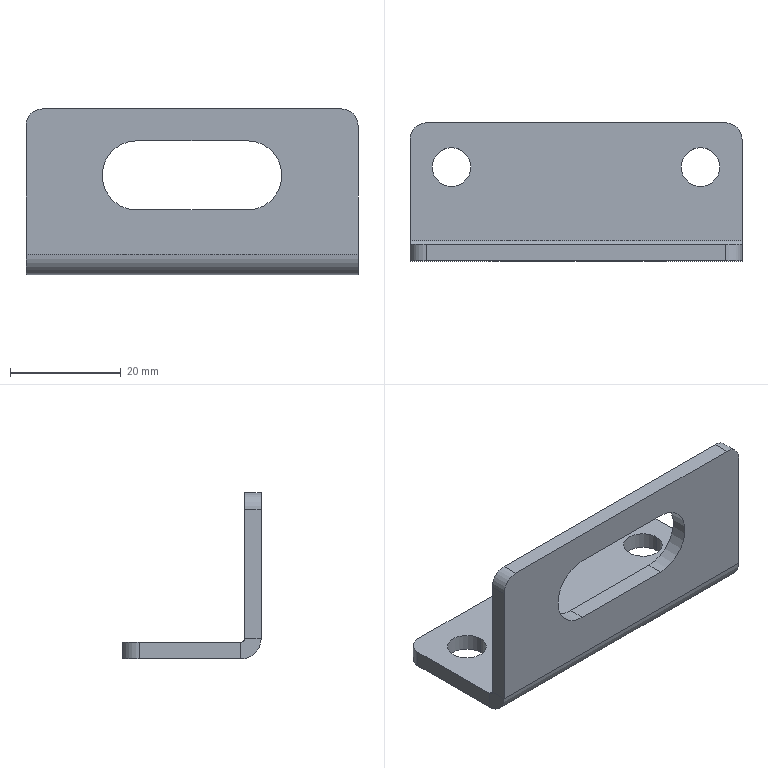Part | SolidWorks | features BaseBody 1 | 1 solid | 26 faces | box 60 x 25 x 30 mm | volume 7815 mm3 | plane 14 | cylinder 12 | commonest cylinder face diameters 6 x4 7 x4 12.5 x2 1.473 x1 7.473 x1
STEP:
#1=CARTESIAN_POINT('',(-26.,4.5,-3.));
#2=VERTEX_POINT('',#1);
#3=CARTESIAN_POINT('',(-19.,4.5,-3.));
#4=VERTEX_POINT('',#3);
#5=CARTESIAN_POINT('',(-22.5,4.5,-3.));
#6=DIRECTION('',(0.,0.,1.));
#7=DIRECTION('',(1.,0.,0.));
#8=AXIS2_PLACEMENT_3D('',#5,#6,#7);
#9=CIRCLE('',#8,3.5);
#10=EDGE_CURVE('',#2,#4,#9,.T.);
#11=ORIENTED_EDGE('',*,*,#10,.F.);
#12=CARTESIAN_POINT('',(-26.,4.5,0.));
#13=VERTEX_POINT('',#12);
#14=CARTESIAN_POINT('',(-26.,4.5,0.));
#15=DIRECTION('',(0.,0.,1.));
#16=VECTOR('',#15,1000.);
#17=LINE('',#14,#16);
#18=EDGE_CURVE('',#2,#13,#17,.T.);
#19=ORIENTED_EDGE('',*,*,#18,.T.);
#20=CARTESIAN_POINT('',(-19.,4.5,0.));
#21=VERTEX_POINT('',#20);
#22=CARTESIAN_POINT('',(-22.5,4.5,0.));
#23=DIRECTION('',(0.,0.,1.));
#24=DIRECTION('',(1.,0.,0.));
#25=AXIS2_PLACEMENT_3D('',#22,#23,#24);
#26=CIRCLE('',#25,3.5);
#27=EDGE_CURVE('',#13,#21,#26,.T.);
#28=ORIENTED_EDGE('',*,*,#27,.T.);
#29=CARTESIAN_POINT('',(-19.,4.5,0.));
#30=DIRECTION('',(0.,0.,1.));
#31=VECTOR('',#30,1000.);
#32=LINE('',#29,#31);
#33=EDGE_CURVE('',#4,#21,#32,.T.);
#34=ORIENTED_EDGE('',*,*,#33,.F.);
#35=EDGE_LOOP('',(#11,#19,#28,#34));
#36=FACE_OUTER_BOUND('',#35,.T.);
#37=CARTESIAN_POINT('',(-22.5,4.5,0.));
#38=DIRECTION('',(0.,0.,1.));
#39=DIRECTION('',(1.,0.,0.));
#40=AXIS2_PLACEMENT_3D('',#37,#38,#39);
#41=CYLINDRICAL_SURFACE('',#40,3.5);
#42=ADVANCED_FACE('',(#36),#41,.F.);
#43=CARTESIAN_POINT('',(19.,4.5,-3.));
#44=VERTEX_POINT('',#43);
#45=CARTESIAN_POINT('',(26.,4.5,-3.));
#46=VERTEX_POINT('',#45);
#47=CARTESIAN_POINT('',(22.5,4.5,-3.));
#48=DIRECTION('',(0.,0.,1.));
#49=DIRECTION('',(1.,0.,0.));
#50=AXIS2_PLACEMENT_3D('',#47,#48,#49);
#51=CIRCLE('',#50,3.5);
#52=EDGE_CURVE('',#44,#46,#51,.T.);
#53=ORIENTED_EDGE('',*,*,#52,.F.);
#54=CARTESIAN_POINT('',(19.,4.5,0.));
#55=VERTEX_POINT('',#54);
#56=CARTESIAN_POINT('',(19.,4.5,0.));
#57=DIRECTION('',(0.,0.,1.));
#58=VECTOR('',#57,1000.);
#59=LINE('',#56,#58);
#60=EDGE_CURVE('',#44,#55,#59,.T.);
#61=ORIENTED_EDGE('',*,*,#60,.T.);
#62=CARTESIAN_POINT('',(26.,4.5,0.));
#63=VERTEX_POINT('',#62);
#64=CARTESIAN_POINT('',(22.5,4.5,0.));
#65=DIRECTION('',(0.,0.,1.));
#66=DIRECTION('',(1.,0.,0.));
#67=AXIS2_PLACEMENT_3D('',#64,#65,#66);
#68=CIRCLE('',#67,3.5);
#69=EDGE_CURVE('',#55,#63,#68,.T.);
#70=ORIENTED_EDGE('',*,*,#69,.T.);
#71=CARTESIAN_POINT('',(26.,4.5,0.));
#72=DIRECTION('',(0.,0.,1.));
#73=VECTOR('',#72,1000.);
#74=LINE('',#71,#73);
#75=EDGE_CURVE('',#46,#63,#74,.T.);
#76=ORIENTED_EDGE('',*,*,#75,.F.);
#77=EDGE_LOOP('',(#53,#61,#70,#76));
#78=FACE_OUTER_BOUND('',#77,.T.);
#79=CARTESIAN_POINT('',(22.5,4.5,0.));
#80=DIRECTION('',(0.,0.,1.));
#81=DIRECTION('',(1.,0.,0.));
#82=AXIS2_PLACEMENT_3D('',#79,#80,#81);
#83=CYLINDRICAL_SURFACE('',#82,3.5);
#84=ADVANCED_FACE('',(#78),#83,.F.);
#85=CARTESIAN_POINT('',(-10.,-9.5,8.75));
#86=VERTEX_POINT('',#85);
#87=CARTESIAN_POINT('',(-10.,-12.5,8.75));
#88=VERTEX_POINT('',#87);
#89=CARTESIAN_POINT('',(-10.,-9.5,8.75));
#90=DIRECTION('',(0.,-1.,0.));
#91=VECTOR('',#90,1000.);
#92=LINE('',#89,#91);
#93=EDGE_CURVE('',#86,#88,#92,.T.);
#94=ORIENTED_EDGE('',*,*,#93,.F.);
#95=CARTESIAN_POINT('',(-10.,-9.5,21.25));
#96=VERTEX_POINT('',#95);
#97=CARTESIAN_POINT('',(-10.,-9.5,15.));
#98=DIRECTION('',(0.,1.,0.));
#99=DIRECTION('',(0.,0.,1.));
#100=AXIS2_PLACEMENT_3D('',#97,#98,#99);
#101=CIRCLE('',#100,6.25);
#102=EDGE_CURVE('',#86,#96,#101,.T.);
#103=ORIENTED_EDGE('',*,*,#102,.T.);
#104=CARTESIAN_POINT('',(-10.,-12.5,21.25));
#105=VERTEX_POINT('',#104);
#106=CARTESIAN_POINT('',(-10.,-9.5,21.25));
#107=DIRECTION('',(0.,-1.,0.));
#108=VECTOR('',#107,1000.);
#109=LINE('',#106,#108);
#110=EDGE_CURVE('',#96,#105,#109,.T.);
#111=ORIENTED_EDGE('',*,*,#110,.T.);
#112=CARTESIAN_POINT('',(-10.,-12.5,15.));
#113=DIRECTION('',(0.,1.,0.));
#114=DIRECTION('',(0.,0.,1.));
#115=AXIS2_PLACEMENT_3D('',#112,#113,#114);
#116=CIRCLE('',#115,6.25);
#117=EDGE_CURVE('',#88,#105,#116,.T.);
#118=ORIENTED_EDGE('',*,*,#117,.F.);
#119=EDGE_LOOP('',(#94,#103,#111,#118));
#120=FACE_OUTER_BOUND('',#119,.T.);
#121=CARTESIAN_POINT('',(-10.,-9.5,15.));
#122=DIRECTION('',(0.,1.,0.));
#123=DIRECTION('',(0.,0.,1.));
#124=AXIS2_PLACEMENT_3D('',#121,#122,#123);
#125=CYLINDRICAL_SURFACE('',#124,6.25);
#126=ADVANCED_FACE('',(#120),#125,.F.);
#127=CARTESIAN_POINT('',(30.,-8.763,-3.));
#128=VERTEX_POINT('',#127);
#129=CARTESIAN_POINT('',(30.,9.5,-3.));
#130=VERTEX_POINT('',#129);
#131=CARTESIAN_POINT('',(30.,12.5,-3.));
#132=DIRECTION('',(0.,1.,0.));
#133=VECTOR('',#132,1000.);
#134=LINE('',#131,#133);
#135=EDGE_CURVE('',#128,#130,#134,.T.);
#136=ORIENTED_EDGE('',*,*,#135,.T.);
#137=CARTESIAN_POINT('',(30.,9.5,0.));
#138=VERTEX_POINT('',#137);
#139=CARTESIAN_POINT('',(30.,9.5,-3.));
#140=DIRECTION('',(0.,0.,1.));
#141=VECTOR('',#140,1000.);
#142=LINE('',#139,#141);
#143=EDGE_CURVE('',#130,#138,#142,.T.);
#144=ORIENTED_EDGE('',*,*,#143,.T.);
#145=CARTESIAN_POINT('',(30.,-8.763,0.));
#146=VERTEX_POINT('',#145);
#147=CARTESIAN_POINT('',(30.,12.5,0.));
#148=DIRECTION('',(0.,1.,0.));
#149=VECTOR('',#148,1000.);
#150=LINE('',#147,#149);
#151=EDGE_CURVE('',#146,#138,#150,.T.);
#152=ORIENTED_EDGE('',*,*,#151,.F.);
#153=CARTESIAN_POINT('',(30.,-8.763,0.));
#154=DIRECTION('',(0.,0.,-1.));
#155=VECTOR('',#154,1000.);
#156=LINE('',#153,#155);
#157=EDGE_CURVE('',#146,#128,#156,.T.);
#158=ORIENTED_EDGE('',*,*,#157,.T.);
#159=EDGE_LOOP('',(#136,#144,#152,#158));
#160=FACE_OUTER_BOUND('',#159,.T.);
#161=CARTESIAN_POINT('',(30.,12.5,-3.));
#162=DIRECTION('',(1.,0.,0.));
#163=DIRECTION('',(0.,1.,0.));
#164=AXIS2_PLACEMENT_3D('',#161,#162,#163);
#165=PLANE('',#164);
#166=ADVANCED_FACE('',(#160),#165,.T.);
#167=CARTESIAN_POINT('',(-22.5,4.5,-3.));
#168=DIRECTION('',(0.,0.,1.));
#169=DIRECTION('',(1.,0.,0.));
#170=AXIS2_PLACEMENT_3D('',#167,#168,#169);
#171=CIRCLE('',#170,3.5);
#172=EDGE_CURVE('',#4,#2,#171,.T.);
#173=ORIENTED_EDGE('',*,*,#172,.T.);
#174=ORIENTED_EDGE('',*,*,#10,.T.);
#175=EDGE_LOOP('',(#173,#174));
#176=FACE_BOUND('',#175,.T.);
#177=CARTESIAN_POINT('',(22.5,4.5,-3.));
#178=DIRECTION('',(0.,0.,1.));
#179=DIRECTION('',(1.,0.,0.));
#180=AXIS2_PLACEMENT_3D('',#177,#178,#179);
#181=CIRCLE('',#180,3.5);
#182=EDGE_CURVE('',#46,#44,#181,.T.);
#183=ORIENTED_EDGE('',*,*,#182,.T.);
#184=ORIENTED_EDGE('',*,*,#52,.T.);
#185=EDGE_LOOP('',(#183,#184));
#186=FACE_BOUND('',#185,.T.);
#187=CARTESIAN_POINT('',(27.,12.5,-3.));
#188=VERTEX_POINT('',#187);
#189=CARTESIAN_POINT('',(-27.,12.5,-3.));
#190=VERTEX_POINT('',#189);
#191=CARTESIAN_POINT('',(-30.,12.5,-3.));
#192=DIRECTION('',(-1.,0.,0.));
#193=VECTOR('',#192,1000.);
#194=LINE('',#191,#193);
#195=EDGE_CURVE('',#188,#190,#194,.T.);
#196=ORIENTED_EDGE('',*,*,#195,.F.);
#197=CARTESIAN_POINT('',(27.,9.5,-3.));
#198=DIRECTION('',(0.,0.,-1.));
#199=DIRECTION('',(1.,0.,0.));
#200=AXIS2_PLACEMENT_3D('',#197,#198,#199);
#201=CIRCLE('',#200,3.);
#202=EDGE_CURVE('',#188,#130,#201,.T.);
#203=ORIENTED_EDGE('',*,*,#202,.T.);
#204=ORIENTED_EDGE('',*,*,#135,.F.);
#205=CARTESIAN_POINT('',(-30.,-8.763,-3.));
#206=VERTEX_POINT('',#205);
#207=CARTESIAN_POINT('',(30.,-8.763,-3.));
#208=DIRECTION('',(-1.,0.,0.));
#209=VECTOR('',#208,1000.);
#210=LINE('',#207,#209);
#211=EDGE_CURVE('',#128,#206,#210,.T.);
#212=ORIENTED_EDGE('',*,*,#211,.T.);
#213=CARTESIAN_POINT('',(-30.,9.5,-3.));
#214=VERTEX_POINT('',#213);
#215=CARTESIAN_POINT('',(-30.,12.5,-3.));
#216=DIRECTION('',(0.,-1.,0.));
#217=VECTOR('',#216,1000.);
#218=LINE('',#215,#217);
#219=EDGE_CURVE('',#214,#206,#218,.T.);
#220=ORIENTED_EDGE('',*,*,#219,.F.);
#221=CARTESIAN_POINT('',(-27.,9.5,-3.));
#222=DIRECTION('',(0.,0.,-1.));
#223=DIRECTION('',(1.,0.,0.));
#224=AXIS2_PLACEMENT_3D('',#221,#222,#223);
#225=CIRCLE('',#224,3.);
#226=EDGE_CURVE('',#214,#190,#225,.T.);
#227=ORIENTED_EDGE('',*,*,#226,.T.);
#228=EDGE_LOOP('',(#196,#203,#204,#212,#220,#227));
#229=FACE_OUTER_BOUND('',#228,.T.);
#230=CARTESIAN_POINT('',(0.,0.,-3.));
#231=DIRECTION('',(0.,0.,1.));
#232=DIRECTION('',(1.,0.,0.));
#233=AXIS2_PLACEMENT_3D('',#230,#231,#232);
#234=PLANE('',#233);
#235=ADVANCED_FACE('',(#176,#186,#229),#234,.F.);
#236=CARTESIAN_POINT('',(-22.5,4.5,0.));
#237=DIRECTION('',(0.,0.,1.));
#238=DIRECTION('',(1.,0.,0.));
#239=AXIS2_PLACEMENT_3D('',#236,#237,#238);
#240=CIRCLE('',#239,3.5);
#241=EDGE_CURVE('',#21,#13,#240,.T.);
#242=ORIENTED_EDGE('',*,*,#241,.F.);
#243=ORIENTED_EDGE('',*,*,#27,.F.);
#244=EDGE_LOOP('',(#242,#243));
#245=FACE_BOUND('',#244,.T.);
#246=CARTESIAN_POINT('',(22.5,4.5,0.));
#247=DIRECTION('',(0.,0.,1.));
#248=DIRECTION('',(1.,0.,0.));
#249=AXIS2_PLACEMENT_3D('',#246,#247,#248);
#250=CIRCLE('',#249,3.5);
#251=EDGE_CURVE('',#63,#55,#250,.T.);
#252=ORIENTED_EDGE('',*,*,#251,.F.);
#253=ORIENTED_EDGE('',*,*,#69,.F.);
#254=EDGE_LOOP('',(#252,#253));
#255=FACE_BOUND('',#254,.T.);
#256=ORIENTED_EDGE('',*,*,#151,.T.);
#257=CARTESIAN_POINT('',(27.,12.5,0.));
#258=VERTEX_POINT('',#257);
#259=CARTESIAN_POINT('',(27.,9.5,0.));
#260=DIRECTION('',(0.,0.,1.));
#261=DIRECTION('',(1.,0.,0.));
#262=AXIS2_PLACEMENT_3D('',#259,#260,#261);
#263=CIRCLE('',#262,3.);
#264=EDGE_CURVE('',#138,#258,#263,.T.);
#265=ORIENTED_EDGE('',*,*,#264,.T.);
#266=CARTESIAN_POINT('',(-27.,12.5,0.));
#267=VERTEX_POINT('',#266);
#268=CARTESIAN_POINT('',(-30.,12.5,0.));
#269=DIRECTION('',(-1.,0.,0.));
#270=VECTOR('',#269,1000.);
#271=LINE('',#268,#270);
#272=EDGE_CURVE('',#258,#267,#271,.T.);
#273=ORIENTED_EDGE('',*,*,#272,.T.);
#274=CARTESIAN_POINT('',(-30.,9.5,0.));
#275=VERTEX_POINT('',#274);
#276=CARTESIAN_POINT('',(-27.,9.5,0.));
#277=DIRECTION('',(0.,0.,1.));
#278=DIRECTION('',(1.,0.,0.));
#279=AXIS2_PLACEMENT_3D('',#276,#277,#278);
#280=CIRCLE('',#279,3.);
#281=EDGE_CURVE('',#267,#275,#280,.T.);
#282=ORIENTED_EDGE('',*,*,#281,.T.);
#283=CARTESIAN_POINT('',(-30.,-8.763,0.));
#284=VERTEX_POINT('',#283);
#285=CARTESIAN_POINT('',(-30.,12.5,0.));
#286=DIRECTION('',(0.,-1.,0.));
#287=VECTOR('',#286,1000.);
#288=LINE('',#285,#287);
#289=EDGE_CURVE('',#275,#284,#288,.T.);
#290=ORIENTED_EDGE('',*,*,#289,.T.);
#291=CARTESIAN_POINT('',(30.,-8.763,0.));
#292=DIRECTION('',(-1.,0.,0.));
#293=VECTOR('',#292,1000.);
#294=LINE('',#291,#293);
#295=EDGE_CURVE('',#146,#284,#294,.T.);
#296=ORIENTED_EDGE('',*,*,#295,.F.);
#297=EDGE_LOOP('',(#256,#265,#273,#282,#290,#296));
#298=FACE_OUTER_BOUND('',#297,.T.);
#299=CARTESIAN_POINT('',(0.,0.,0.));
#300=DIRECTION('',(0.,0.,1.));
#301=DIRECTION('',(1.,0.,0.));
#302=AXIS2_PLACEMENT_3D('',#299,#300,#301);
#303=PLANE('',#302);
#304=ADVANCED_FACE('',(#245,#255,#298),#303,.T.);
#305=ORIENTED_EDGE('',*,*,#289,.F.);
#306=CARTESIAN_POINT('',(-30.,9.5,-3.));
#307=DIRECTION('',(0.,0.,-1.));
#308=VECTOR('',#307,1000.);
#309=LINE('',#306,#308);
#310=EDGE_CURVE('',#275,#214,#309,.T.);
#311=ORIENTED_EDGE('',*,*,#310,.T.);
#312=ORIENTED_EDGE('',*,*,#219,.T.);
#313=CARTESIAN_POINT('',(-30.,-8.763,0.));
#314=DIRECTION('',(0.,0.,-1.));
#315=VECTOR('',#314,1000.);
#316=LINE('',#313,#315);
#317=EDGE_CURVE('',#284,#206,#316,.T.);
#318=ORIENTED_EDGE('',*,*,#317,.F.);
#319=EDGE_LOOP('',(#305,#311,#312,#318));
#320=FACE_OUTER_BOUND('',#319,.T.);
#321=CARTESIAN_POINT('',(-30.,12.5,-3.));
#322=DIRECTION('',(-1.,0.,0.));
#323=DIRECTION('',(0.,-1.,0.));
#324=AXIS2_PLACEMENT_3D('',#321,#322,#323);
#325=PLANE('',#324);
#326=ADVANCED_FACE('',(#320),#325,.T.);
#327=ORIENTED_EDGE('',*,*,#272,.F.);
#328=CARTESIAN_POINT('',(27.,12.5,-3.));
#329=DIRECTION('',(0.,0.,-1.));
#330=VECTOR('',#329,1000.);
#331=LINE('',#328,#330);
#332=EDGE_CURVE('',#258,#188,#331,.T.);
#333=ORIENTED_EDGE('',*,*,#332,.T.);
#334=ORIENTED_EDGE('',*,*,#195,.T.);
#335=CARTESIAN_POINT('',(-27.,12.5,-3.));
#336=DIRECTION('',(0.,0.,1.));
#337=VECTOR('',#336,1000.);
#338=LINE('',#335,#337);
#339=EDGE_CURVE('',#190,#267,#338,.T.);
#340=ORIENTED_EDGE('',*,*,#339,.T.);
#341=EDGE_LOOP('',(#327,#333,#334,#340));
#342=FACE_OUTER_BOUND('',#341,.T.);
#343=CARTESIAN_POINT('',(-30.,12.5,-3.));
#344=DIRECTION('',(0.,1.,0.));
#345=DIRECTION('',(0.,0.,1.));
#346=AXIS2_PLACEMENT_3D('',#343,#344,#345);
#347=PLANE('',#346);
#348=ADVANCED_FACE('',(#342),#347,.T.);
#349=CARTESIAN_POINT('',(-30.,-9.5,0.7366));
#350=VERTEX_POINT('',#349);
#351=CARTESIAN_POINT('',(-30.,-12.5,0.7366));
#352=VERTEX_POINT('',#351);
#353=CARTESIAN_POINT('',(-30.,-12.5,0.7366));
#354=DIRECTION('',(0.,-1.,0.));
#355=VECTOR('',#354,1000.);
#356=LINE('',#353,#355);
#357=EDGE_CURVE('',#350,#352,#356,.T.);
#358=ORIENTED_EDGE('',*,*,#357,.F.);
#359=CARTESIAN_POINT('',(-30.,-8.763,0.7366));
#360=DIRECTION('',(-1.,0.,0.));
#361=DIRECTION('',(0.,0.,-1.));
#362=AXIS2_PLACEMENT_3D('',#359,#360,#361);
#363=CIRCLE('',#362,0.7366);
#364=EDGE_CURVE('',#284,#350,#363,.T.);
#365=ORIENTED_EDGE('',*,*,#364,.F.);
#366=ORIENTED_EDGE('',*,*,#317,.T.);
#367=CARTESIAN_POINT('',(-30.,-8.763,0.7366));
#368=DIRECTION('',(-1.,0.,0.));
#369=DIRECTION('',(0.,0.,-1.));
#370=AXIS2_PLACEMENT_3D('',#367,#368,#369);
#371=CIRCLE('',#370,3.737);
#372=EDGE_CURVE('',#206,#352,#371,.T.);
#373=ORIENTED_EDGE('',*,*,#372,.T.);
#374=EDGE_LOOP('',(#358,#365,#366,#373));
#375=FACE_OUTER_BOUND('',#374,.T.);
#376=CARTESIAN_POINT('',(-30.,-8.763,0.7366));
#377=DIRECTION('',(-1.,0.,0.));
#378=DIRECTION('',(0.,0.,1.));
#379=AXIS2_PLACEMENT_3D('',#376,#377,#378);
#380=PLANE('',#379);
#381=ADVANCED_FACE('',(#375),#380,.T.);
#382=CARTESIAN_POINT('',(30.,-9.5,0.7366));
#383=VERTEX_POINT('',#382);
#384=CARTESIAN_POINT('',(30.,-8.763,0.7366));
#385=DIRECTION('',(1.,0.,0.));
#386=DIRECTION('',(0.,0.,-1.));
#387=AXIS2_PLACEMENT_3D('',#384,#385,#386);
#388=CIRCLE('',#387,0.7366);
#389=EDGE_CURVE('',#383,#146,#388,.T.);
#390=ORIENTED_EDGE('',*,*,#389,.F.);
#391=CARTESIAN_POINT('',(30.,-12.5,0.7366));
#392=VERTEX_POINT('',#391);
#393=CARTESIAN_POINT('',(30.,-9.5,0.7366));
#394=DIRECTION('',(0.,-1.,0.));
#395=VECTOR('',#394,1000.);
#396=LINE('',#393,#395);
#397=EDGE_CURVE('',#383,#392,#396,.T.);
#398=ORIENTED_EDGE('',*,*,#397,.T.);
#399=CARTESIAN_POINT('',(30.,-8.763,0.7366));
#400=DIRECTION('',(1.,0.,0.));
#401=DIRECTION('',(0.,0.,-1.));
#402=AXIS2_PLACEMENT_3D('',#399,#400,#401);
#403=CIRCLE('',#402,3.737);
#404=EDGE_CURVE('',#392,#128,#403,.T.);
#405=ORIENTED_EDGE('',*,*,#404,.T.);
#406=ORIENTED_EDGE('',*,*,#157,.F.);
#407=EDGE_LOOP('',(#390,#398,#405,#406));
#408=FACE_OUTER_BOUND('',#407,.T.);
#409=CARTESIAN_POINT('',(30.,-8.763,0.7366));
#410=DIRECTION('',(-1.,0.,0.));
#411=DIRECTION('',(0.,0.,1.));
#412=AXIS2_PLACEMENT_3D('',#409,#410,#411);
#413=PLANE('',#412);
#414=ADVANCED_FACE('',(#408),#413,.F.);
#415=ORIENTED_EDGE('',*,*,#211,.F.);
#416=ORIENTED_EDGE('',*,*,#404,.F.);
#417=CARTESIAN_POINT('',(-30.,-12.5,0.7366));
#418=DIRECTION('',(-1.,0.,0.));
#419=VECTOR('',#418,1000.);
#420=LINE('',#417,#419);
#421=EDGE_CURVE('',#392,#352,#420,.T.);
#422=ORIENTED_EDGE('',*,*,#421,.T.);
#423=ORIENTED_EDGE('',*,*,#372,.F.);
#424=EDGE_LOOP('',(#415,#416,#422,#423));
#425=FACE_OUTER_BOUND('',#424,.T.);
#426=CARTESIAN_POINT('',(30.,-8.763,0.7366));
#427=DIRECTION('',(1.,0.,0.));
#428=DIRECTION('',(0.,-1.,0.));
#429=AXIS2_PLACEMENT_3D('',#426,#427,#428);
#430=CYLINDRICAL_SURFACE('',#429,3.737);
#431=ADVANCED_FACE('',(#425),#430,.T.);
#432=ORIENTED_EDGE('',*,*,#295,.T.);
#433=ORIENTED_EDGE('',*,*,#364,.T.);
#434=CARTESIAN_POINT('',(-30.,-9.5,0.7366));
#435=DIRECTION('',(1.,0.,0.));
#436=VECTOR('',#435,1000.);
#437=LINE('',#434,#436);
#438=EDGE_CURVE('',#350,#383,#437,.T.);
#439=ORIENTED_EDGE('',*,*,#438,.T.);
#440=ORIENTED_EDGE('',*,*,#389,.T.);
#441=EDGE_LOOP('',(#432,#433,#439,#440));
#442=FACE_OUTER_BOUND('',#441,.T.);
#443=CARTESIAN_POINT('',(30.,-8.763,0.7366));
#444=DIRECTION('',(1.,0.,0.));
#445=DIRECTION('',(0.,-1.,0.));
#446=AXIS2_PLACEMENT_3D('',#443,#444,#445);
#447=CYLINDRICAL_SURFACE('',#446,0.7366);
#448=ADVANCED_FACE('',(#442),#447,.F.);
#449=CARTESIAN_POINT('',(-30.,-12.5,24.));
#450=VERTEX_POINT('',#449);
#451=CARTESIAN_POINT('',(-30.,-12.5,0.));
#452=DIRECTION('',(0.,0.,-1.));
#453=VECTOR('',#452,1000.);
#454=LINE('',#451,#453);
#455=EDGE_CURVE('',#450,#352,#454,.T.);
#456=ORIENTED_EDGE('',*,*,#455,.F.);
#457=CARTESIAN_POINT('',(-30.,-9.5,24.));
#458=VERTEX_POINT('',#457);
#459=CARTESIAN_POINT('',(-30.,-12.5,24.));
#460=DIRECTION('',(0.,1.,0.));
#461=VECTOR('',#460,1000.);
#462=LINE('',#459,#461);
#463=EDGE_CURVE('',#450,#458,#462,.T.);
#464=ORIENTED_EDGE('',*,*,#463,.T.);
#465=CARTESIAN_POINT('',(-30.,-9.5,0.));
#466=DIRECTION('',(0.,0.,-1.));
#467=VECTOR('',#466,1000.);
#468=LINE('',#465,#467);
#469=EDGE_CURVE('',#458,#350,#468,.T.);
#470=ORIENTED_EDGE('',*,*,#469,.T.);
#471=ORIENTED_EDGE('',*,*,#357,.T.);
#472=EDGE_LOOP('',(#456,#464,#470,#471));
#473=FACE_OUTER_BOUND('',#472,.T.);
#474=CARTESIAN_POINT('',(-30.,-12.5,0.));
#475=DIRECTION('',(1.,0.,0.));
#476=DIRECTION('',(0.,0.,-1.));
#477=AXIS2_PLACEMENT_3D('',#474,#475,#476);
#478=PLANE('',#477);
#479=ADVANCED_FACE('',(#473),#478,.F.);
#480=CARTESIAN_POINT('',(30.,-9.5,24.));
#481=VERTEX_POINT('',#480);
#482=CARTESIAN_POINT('',(30.,-9.5,27.));
#483=DIRECTION('',(0.,0.,1.));
#484=VECTOR('',#483,1000.);
#485=LINE('',#482,#484);
#486=EDGE_CURVE('',#383,#481,#485,.T.);
#487=ORIENTED_EDGE('',*,*,#486,.T.);
#488=CARTESIAN_POINT('',(30.,-12.5,24.));
#489=VERTEX_POINT('',#488);
#490=CARTESIAN_POINT('',(30.,-12.5,24.));
#491=DIRECTION('',(0.,-1.,0.));
#492=VECTOR('',#491,1000.);
#493=LINE('',#490,#492);
#494=EDGE_CURVE('',#481,#489,#493,.T.);
#495=ORIENTED_EDGE('',*,*,#494,.T.);
#496=CARTESIAN_POINT('',(30.,-12.5,0.));
#497=DIRECTION('',(0.,0.,1.));
#498=VECTOR('',#497,1000.);
#499=LINE('',#496,#498);
#500=EDGE_CURVE('',#392,#489,#499,.T.);
#501=ORIENTED_EDGE('',*,*,#500,.F.);
#502=ORIENTED_EDGE('',*,*,#397,.F.);
#503=EDGE_LOOP('',(#487,#495,#501,#502));
#504=FACE_OUTER_BOUND('',#503,.T.);
#505=CARTESIAN_POINT('',(30.,-12.5,27.));
#506=DIRECTION('',(-1.,0.,0.));
#507=DIRECTION('',(0.,0.,1.));
#508=AXIS2_PLACEMENT_3D('',#505,#506,#507);
#509=PLANE('',#508);
#510=ADVANCED_FACE('',(#504),#509,.F.);
#511=CARTESIAN_POINT('',(10.,-12.5,21.25));
#512=VERTEX_POINT('',#511);
#513=CARTESIAN_POINT('',(10.,-12.5,8.75));
#514=VERTEX_POINT('',#513);
#515=CARTESIAN_POINT('',(10.,-12.5,15.));
#516=DIRECTION('',(0.,1.,0.));
#517=DIRECTION('',(0.,0.,1.));
#518=AXIS2_PLACEMENT_3D('',#515,#516,#517);
#519=CIRCLE('',#518,6.25);
#520=EDGE_CURVE('',#512,#514,#519,.T.);
#521=ORIENTED_EDGE('',*,*,#520,.T.);
#522=CARTESIAN_POINT('',(0.,-12.5,8.75));
#523=DIRECTION('',(-1.,0.,0.));
#524=VECTOR('',#523,1000.);
#525=LINE('',#522,#524);
#526=EDGE_CURVE('',#514,#88,#525,.T.);
#527=ORIENTED_EDGE('',*,*,#526,.T.);
#528=ORIENTED_EDGE('',*,*,#117,.T.);
#529=CARTESIAN_POINT('',(0.,-12.5,21.25));
#530=DIRECTION('',(1.,0.,0.));
#531=VECTOR('',#530,1000.);
#532=LINE('',#529,#531);
#533=EDGE_CURVE('',#105,#512,#532,.T.);
#534=ORIENTED_EDGE('',*,*,#533,.T.);
#535=EDGE_LOOP('',(#521,#527,#528,#534));
#536=FACE_BOUND('',#535,.T.);
#537=CARTESIAN_POINT('',(27.,-12.5,27.));
#538=VERTEX_POINT('',#537);
#539=CARTESIAN_POINT('',(-27.,-12.5,27.));
#540=VERTEX_POINT('',#539);
#541=CARTESIAN_POINT('',(0.,-12.5,27.));
#542=DIRECTION('',(-1.,0.,0.));
#543=VECTOR('',#542,1000.);
#544=LINE('',#541,#543);
#545=EDGE_CURVE('',#538,#540,#544,.T.);
#546=ORIENTED_EDGE('',*,*,#545,.T.);
#547=CARTESIAN_POINT('',(-27.,-12.5,24.));
#548=DIRECTION('',(0.,-1.,0.));
#549=DIRECTION('',(0.,0.,1.));
#550=AXIS2_PLACEMENT_3D('',#547,#548,#549);
#551=CIRCLE('',#550,3.);
#552=EDGE_CURVE('',#540,#450,#551,.T.);
#553=ORIENTED_EDGE('',*,*,#552,.T.);
#554=ORIENTED_EDGE('',*,*,#455,.T.);
#555=ORIENTED_EDGE('',*,*,#421,.F.);
#556=ORIENTED_EDGE('',*,*,#500,.T.);
#557=CARTESIAN_POINT('',(27.,-12.5,24.));
#558=DIRECTION('',(0.,-1.,0.));
#559=DIRECTION('',(0.,0.,1.));
#560=AXIS2_PLACEMENT_3D('',#557,#558,#559);
#561=CIRCLE('',#560,3.);
#562=EDGE_CURVE('',#489,#538,#561,.T.);
#563=ORIENTED_EDGE('',*,*,#562,.T.);
#564=EDGE_LOOP('',(#546,#553,#554,#555,#556,#563));
#565=FACE_OUTER_BOUND('',#564,.T.);
#566=CARTESIAN_POINT('',(0.,-12.5,0.));
#567=DIRECTION('',(0.,1.,0.));
#568=DIRECTION('',(0.,0.,1.));
#569=AXIS2_PLACEMENT_3D('',#566,#567,#568);
#570=PLANE('',#569);
#571=ADVANCED_FACE('',(#536,#565),#570,.F.);
#572=CARTESIAN_POINT('',(10.,-9.5,8.75));
#573=VERTEX_POINT('',#572);
#574=CARTESIAN_POINT('',(-10.,-9.5,8.75));
#575=DIRECTION('',(-1.,0.,0.));
#576=VECTOR('',#575,1000.);
#577=LINE('',#574,#576);
#578=EDGE_CURVE('',#573,#86,#577,.T.);
#579=ORIENTED_EDGE('',*,*,#578,.F.);
#580=CARTESIAN_POINT('',(10.,-9.5,21.25));
#581=VERTEX_POINT('',#580);
#582=CARTESIAN_POINT('',(10.,-9.5,15.));
#583=DIRECTION('',(0.,1.,0.));
#584=DIRECTION('',(0.,0.,1.));
#585=AXIS2_PLACEMENT_3D('',#582,#583,#584);
#586=CIRCLE('',#585,6.25);
#587=EDGE_CURVE('',#581,#573,#586,.T.);
#588=ORIENTED_EDGE('',*,*,#587,.F.);
#589=CARTESIAN_POINT('',(-10.,-9.5,21.25));
#590=DIRECTION('',(1.,0.,0.));
#591=VECTOR('',#590,1000.);
#592=LINE('',#589,#591);
#593=EDGE_CURVE('',#96,#581,#592,.T.);
#594=ORIENTED_EDGE('',*,*,#593,.F.);
#595=ORIENTED_EDGE('',*,*,#102,.F.);
#596=EDGE_LOOP('',(#579,#588,#594,#595));
#597=FACE_BOUND('',#596,.T.);
#598=ORIENTED_EDGE('',*,*,#469,.F.);
#599=CARTESIAN_POINT('',(-27.,-9.5,27.));
#600=VERTEX_POINT('',#599);
#601=CARTESIAN_POINT('',(-27.,-9.5,24.));
#602=DIRECTION('',(0.,1.,0.));
#603=DIRECTION('',(0.,0.,1.));
#604=AXIS2_PLACEMENT_3D('',#601,#602,#603);
#605=CIRCLE('',#604,3.);
#606=EDGE_CURVE('',#458,#600,#605,.T.);
#607=ORIENTED_EDGE('',*,*,#606,.T.);
#608=CARTESIAN_POINT('',(27.,-9.5,27.));
#609=VERTEX_POINT('',#608);
#610=CARTESIAN_POINT('',(-30.,-9.5,27.));
#611=DIRECTION('',(-1.,0.,0.));
#612=VECTOR('',#611,1000.);
#613=LINE('',#610,#612);
#614=EDGE_CURVE('',#609,#600,#613,.T.);
#615=ORIENTED_EDGE('',*,*,#614,.F.);
#616=CARTESIAN_POINT('',(27.,-9.5,24.));
#617=DIRECTION('',(0.,1.,0.));
#618=DIRECTION('',(0.,0.,1.));
#619=AXIS2_PLACEMENT_3D('',#616,#617,#618);
#620=CIRCLE('',#619,3.);
#621=EDGE_CURVE('',#609,#481,#620,.T.);
#622=ORIENTED_EDGE('',*,*,#621,.T.);
#623=ORIENTED_EDGE('',*,*,#486,.F.);
#624=ORIENTED_EDGE('',*,*,#438,.F.);
#625=EDGE_LOOP('',(#598,#607,#615,#622,#623,#624));
#626=FACE_OUTER_BOUND('',#625,.T.);
#627=CARTESIAN_POINT('',(0.,-9.5,0.));
#628=DIRECTION('',(0.,1.,0.));
#629=DIRECTION('',(0.,0.,1.));
#630=AXIS2_PLACEMENT_3D('',#627,#628,#629);
#631=PLANE('',#630);
#632=ADVANCED_FACE('',(#597,#626),#631,.T.);
#633=ORIENTED_EDGE('',*,*,#614,.T.);
#634=CARTESIAN_POINT('',(-27.,-12.5,27.));
#635=DIRECTION('',(0.,-1.,0.));
#636=VECTOR('',#635,1000.);
#637=LINE('',#634,#636);
#638=EDGE_CURVE('',#600,#540,#637,.T.);
#639=ORIENTED_EDGE('',*,*,#638,.T.);
#640=ORIENTED_EDGE('',*,*,#545,.F.);
#641=CARTESIAN_POINT('',(27.,-12.5,27.));
#642=DIRECTION('',(0.,1.,0.));
#643=VECTOR('',#642,1000.);
#644=LINE('',#641,#643);
#645=EDGE_CURVE('',#538,#609,#644,.T.);
#646=ORIENTED_EDGE('',*,*,#645,.T.);
#647=EDGE_LOOP('',(#633,#639,#640,#646));
#648=FACE_OUTER_BOUND('',#647,.T.);
#649=CARTESIAN_POINT('',(-30.,-12.5,27.));
#650=DIRECTION('',(0.,0.,-1.));
#651=DIRECTION('',(0.,1.,0.));
#652=AXIS2_PLACEMENT_3D('',#649,#650,#651);
#653=PLANE('',#652);
#654=ADVANCED_FACE('',(#648),#653,.F.);
#655=ORIENTED_EDGE('',*,*,#60,.F.);
#656=ORIENTED_EDGE('',*,*,#182,.F.);
#657=ORIENTED_EDGE('',*,*,#75,.T.);
#658=ORIENTED_EDGE('',*,*,#251,.T.);
#659=EDGE_LOOP('',(#655,#656,#657,#658));
#660=FACE_OUTER_BOUND('',#659,.T.);
#661=CARTESIAN_POINT('',(22.5,4.5,0.));
#662=DIRECTION('',(0.,0.,1.));
#663=DIRECTION('',(1.,0.,0.));
#664=AXIS2_PLACEMENT_3D('',#661,#662,#663);
#665=CYLINDRICAL_SURFACE('',#664,3.5);
#666=ADVANCED_FACE('',(#660),#665,.F.);
#667=ORIENTED_EDGE('',*,*,#18,.F.);
#668=ORIENTED_EDGE('',*,*,#172,.F.);
#669=ORIENTED_EDGE('',*,*,#33,.T.);
#670=ORIENTED_EDGE('',*,*,#241,.T.);
#671=EDGE_LOOP('',(#667,#668,#669,#670));
#672=FACE_OUTER_BOUND('',#671,.T.);
#673=CARTESIAN_POINT('',(-22.5,4.5,0.));
#674=DIRECTION('',(0.,0.,1.));
#675=DIRECTION('',(1.,0.,0.));
#676=AXIS2_PLACEMENT_3D('',#673,#674,#675);
#677=CYLINDRICAL_SURFACE('',#676,3.5);
#678=ADVANCED_FACE('',(#672),#677,.F.);
#679=ORIENTED_EDGE('',*,*,#587,.T.);
#680=CARTESIAN_POINT('',(10.,-19.5,8.75));
#681=DIRECTION('',(0.,1.,0.));
#682=VECTOR('',#681,1000.);
#683=LINE('',#680,#682);
#684=EDGE_CURVE('',#514,#573,#683,.T.);
#685=ORIENTED_EDGE('',*,*,#684,.F.);
#686=ORIENTED_EDGE('',*,*,#520,.F.);
#687=CARTESIAN_POINT('',(10.,-19.5,21.25));
#688=DIRECTION('',(0.,1.,0.));
#689=VECTOR('',#688,1000.);
#690=LINE('',#687,#689);
#691=EDGE_CURVE('',#512,#581,#690,.T.);
#692=ORIENTED_EDGE('',*,*,#691,.T.);
#693=EDGE_LOOP('',(#679,#685,#686,#692));
#694=FACE_OUTER_BOUND('',#693,.T.);
#695=CARTESIAN_POINT('',(10.,-9.5,15.));
#696=DIRECTION('',(0.,1.,0.));
#697=DIRECTION('',(0.,0.,1.));
#698=AXIS2_PLACEMENT_3D('',#695,#696,#697);
#699=CYLINDRICAL_SURFACE('',#698,6.25);
#700=ADVANCED_FACE('',(#694),#699,.F.);
#701=ORIENTED_EDGE('',*,*,#110,.F.);
#702=ORIENTED_EDGE('',*,*,#593,.T.);
#703=ORIENTED_EDGE('',*,*,#691,.F.);
#704=ORIENTED_EDGE('',*,*,#533,.F.);
#705=EDGE_LOOP('',(#701,#702,#703,#704));
#706=FACE_OUTER_BOUND('',#705,.T.);
#707=CARTESIAN_POINT('',(-10.,-19.5,21.25));
#708=DIRECTION('',(0.,0.,1.));
#709=DIRECTION('',(0.,-1.,0.));
#710=AXIS2_PLACEMENT_3D('',#707,#708,#709);
#711=PLANE('',#710);
#712=ADVANCED_FACE('',(#706),#711,.F.);
#713=ORIENTED_EDGE('',*,*,#684,.T.);
#714=ORIENTED_EDGE('',*,*,#578,.T.);
#715=ORIENTED_EDGE('',*,*,#93,.T.);
#716=ORIENTED_EDGE('',*,*,#526,.F.);
#717=EDGE_LOOP('',(#713,#714,#715,#716));
#718=FACE_OUTER_BOUND('',#717,.T.);
#719=CARTESIAN_POINT('',(-10.,-19.5,8.75));
#720=DIRECTION('',(0.,0.,-1.));
#721=DIRECTION('',(0.,1.,0.));
#722=AXIS2_PLACEMENT_3D('',#719,#720,#721);
#723=PLANE('',#722);
#724=ADVANCED_FACE('',(#718),#723,.F.);
#725=ORIENTED_EDGE('',*,*,#552,.F.);
#726=ORIENTED_EDGE('',*,*,#638,.F.);
#727=ORIENTED_EDGE('',*,*,#606,.F.);
#728=ORIENTED_EDGE('',*,*,#463,.F.);
#729=EDGE_LOOP('',(#725,#726,#727,#728));
#730=FACE_OUTER_BOUND('',#729,.T.);
#731=CARTESIAN_POINT('',(-27.,-12.5,24.));
#732=DIRECTION('',(0.,1.,0.));
#733=DIRECTION('',(0.,0.,1.));
#734=AXIS2_PLACEMENT_3D('',#731,#732,#733);
#735=CYLINDRICAL_SURFACE('',#734,3.);
#736=ADVANCED_FACE('',(#730),#735,.T.);
#737=ORIENTED_EDGE('',*,*,#562,.F.);
#738=ORIENTED_EDGE('',*,*,#494,.F.);
#739=ORIENTED_EDGE('',*,*,#621,.F.);
#740=ORIENTED_EDGE('',*,*,#645,.F.);
#741=EDGE_LOOP('',(#737,#738,#739,#740));
#742=FACE_OUTER_BOUND('',#741,.T.);
#743=CARTESIAN_POINT('',(27.,-12.5,24.));
#744=DIRECTION('',(0.,1.,0.));
#745=DIRECTION('',(0.,0.,1.));
#746=AXIS2_PLACEMENT_3D('',#743,#744,#745);
#747=CYLINDRICAL_SURFACE('',#746,3.);
#748=ADVANCED_FACE('',(#742),#747,.T.);
#749=ORIENTED_EDGE('',*,*,#202,.F.);
#750=ORIENTED_EDGE('',*,*,#332,.F.);
#751=ORIENTED_EDGE('',*,*,#264,.F.);
#752=ORIENTED_EDGE('',*,*,#143,.F.);
#753=EDGE_LOOP('',(#749,#750,#751,#752));
#754=FACE_OUTER_BOUND('',#753,.T.);
#755=CARTESIAN_POINT('',(27.,9.5,-3.));
#756=DIRECTION('',(0.,0.,1.));
#757=DIRECTION('',(1.,0.,0.));
#758=AXIS2_PLACEMENT_3D('',#755,#756,#757);
#759=CYLINDRICAL_SURFACE('',#758,3.);
#760=ADVANCED_FACE('',(#754),#759,.T.);
#761=ORIENTED_EDGE('',*,*,#226,.F.);
#762=ORIENTED_EDGE('',*,*,#310,.F.);
#763=ORIENTED_EDGE('',*,*,#281,.F.);
#764=ORIENTED_EDGE('',*,*,#339,.F.);
#765=EDGE_LOOP('',(#761,#762,#763,#764));
#766=FACE_OUTER_BOUND('',#765,.T.);
#767=CARTESIAN_POINT('',(-27.,9.5,-3.));
#768=DIRECTION('',(0.,0.,1.));
#769=DIRECTION('',(1.,0.,0.));
#770=AXIS2_PLACEMENT_3D('',#767,#768,#769);
#771=CYLINDRICAL_SURFACE('',#770,3.);
#772=ADVANCED_FACE('',(#766),#771,.T.);
#773=CLOSED_SHELL('',(#42,#84,#126,#166,#235,#304,#326,#348,#381,#414,#431,#448,#479,#510,#571,#632,#654,#666,#678,#700,#712,#724,#736,#748,#760,#772));
#774=MANIFOLD_SOLID_BREP('',#773);
#775=CARTESIAN_POINT('',(0.,0.,0.));
#776=DIRECTION('',(0.,0.,1.));
#777=DIRECTION('',(1.,0.,0.));
#778=AXIS2_PLACEMENT_3D('',#775,#776,#777);
#779=(LENGTH_UNIT()NAMED_UNIT(*)SI_UNIT(.MILLI.,.METRE.));
#780=UNCERTAINTY_MEASURE_WITH_UNIT(LENGTH_MEASURE(0.00001),#779,'','');
#781=(NAMED_UNIT(*)PLANE_ANGLE_UNIT()SI_UNIT($,.RADIAN.));
#782=(NAMED_UNIT(*)SI_UNIT($,.STERADIAN.)SOLID_ANGLE_UNIT());
#783=(GEOMETRIC_REPRESENTATION_CONTEXT(3)GLOBAL_UNCERTAINTY_ASSIGNED_CONTEXT((#780))GLOBAL_UNIT_ASSIGNED_CONTEXT((#779,#781,#782))REPRESENTATION_CONTEXT('',''));
#784=ADVANCED_BREP_SHAPE_REPRESENTATION('',(#774,#778),#783);